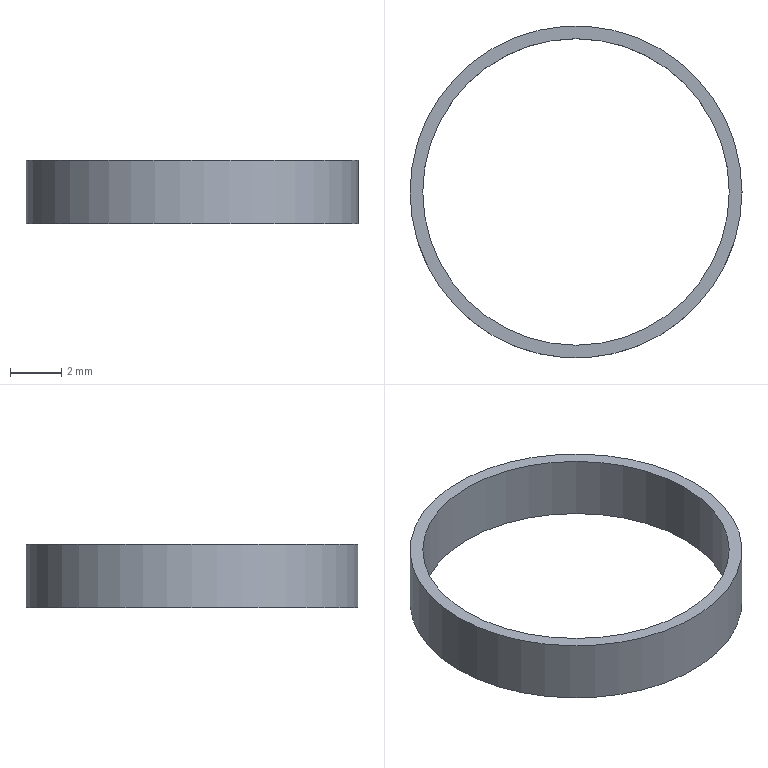Part | STEP file | lll_id1134_x_t | 1 solid | 4 faces | box 13 x 13 x 2.5 mm | volume 49.087 mm3 | cylinder 2 | plane 2 | commonest cylinder face diameters 12 x1 13 x1
STEP:
#1=CARTESIAN_POINT('',(383.,-100.,-0.15));
#2=VERTEX_POINT('',#1);
#3=CARTESIAN_POINT('',(389.5,-100.,-0.15));
#4=DIRECTION('',(0.,0.,1.));
#5=DIRECTION('',(-1.,0.,0.));
#6=AXIS2_PLACEMENT_3D('',#3,#4,#5);
#7=CIRCLE('',#6,6.5);
#8=EDGE_CURVE('',#2,#2,#7,.T.);
#9=ORIENTED_EDGE('',*,*,#8,.T.);
#10=EDGE_LOOP('',(#9));
#11=FACE_BOUND('',#10,.T.);
#12=CARTESIAN_POINT('',(383.,-100.,2.35));
#13=VERTEX_POINT('',#12);
#14=CARTESIAN_POINT('',(389.5,-100.,2.35));
#15=DIRECTION('',(0.,0.,1.));
#16=DIRECTION('',(-1.,0.,0.));
#17=AXIS2_PLACEMENT_3D('',#14,#15,#16);
#18=CIRCLE('',#17,6.5);
#19=EDGE_CURVE('',#13,#13,#18,.T.);
#20=ORIENTED_EDGE('',*,*,#19,.F.);
#21=EDGE_LOOP('',(#20));
#22=FACE_BOUND('',#21,.T.);
#23=CARTESIAN_POINT('',(389.5,-100.,-0.15));
#24=DIRECTION('',(0.,0.,1.));
#25=DIRECTION('',(1.,0.,0.));
#26=AXIS2_PLACEMENT_3D('',#23,#24,#25);
#27=CYLINDRICAL_SURFACE('',#26,6.5);
#28=ADVANCED_FACE('',(#11,#22),#27,.T.);
#29=CARTESIAN_POINT('',(383.5,-100.,-0.15));
#30=VERTEX_POINT('',#29);
#31=CARTESIAN_POINT('',(389.5,-100.,-0.15));
#32=DIRECTION('',(0.,0.,1.));
#33=DIRECTION('',(-1.,0.,0.));
#34=AXIS2_PLACEMENT_3D('',#31,#32,#33);
#35=CIRCLE('',#34,6.);
#36=EDGE_CURVE('',#30,#30,#35,.T.);
#37=ORIENTED_EDGE('',*,*,#36,.F.);
#38=EDGE_LOOP('',(#37));
#39=FACE_BOUND('',#38,.T.);
#40=CARTESIAN_POINT('',(383.5,-100.,2.35));
#41=VERTEX_POINT('',#40);
#42=CARTESIAN_POINT('',(389.5,-100.,2.35));
#43=DIRECTION('',(0.,0.,1.));
#44=DIRECTION('',(-1.,0.,0.));
#45=AXIS2_PLACEMENT_3D('',#42,#43,#44);
#46=CIRCLE('',#45,6.);
#47=EDGE_CURVE('',#41,#41,#46,.T.);
#48=ORIENTED_EDGE('',*,*,#47,.T.);
#49=EDGE_LOOP('',(#48));
#50=FACE_BOUND('',#49,.T.);
#51=CARTESIAN_POINT('',(389.5,-100.,-0.15));
#52=DIRECTION('',(0.,0.,1.));
#53=DIRECTION('',(1.,0.,0.));
#54=AXIS2_PLACEMENT_3D('',#51,#52,#53);
#55=CYLINDRICAL_SURFACE('',#54,6.);
#56=ADVANCED_FACE('',(#39,#50),#55,.F.);
#57=ORIENTED_EDGE('',*,*,#8,.F.);
#58=EDGE_LOOP('',(#57));
#59=FACE_BOUND('',#58,.T.);
#60=ORIENTED_EDGE('',*,*,#36,.T.);
#61=EDGE_LOOP('',(#60));
#62=FACE_BOUND('',#61,.T.);
#63=CARTESIAN_POINT('',(389.5,-100.,-0.15));
#64=DIRECTION('',(0.,0.,1.));
#65=DIRECTION('',(1.,0.,0.));
#66=AXIS2_PLACEMENT_3D('',#63,#64,#65);
#67=PLANE('',#66);
#68=ADVANCED_FACE('',(#59,#62),#67,.F.);
#69=ORIENTED_EDGE('',*,*,#19,.T.);
#70=EDGE_LOOP('',(#69));
#71=FACE_BOUND('',#70,.T.);
#72=ORIENTED_EDGE('',*,*,#47,.F.);
#73=EDGE_LOOP('',(#72));
#74=FACE_BOUND('',#73,.T.);
#75=CARTESIAN_POINT('',(389.5,-100.,2.35));
#76=DIRECTION('',(0.,0.,1.));
#77=DIRECTION('',(1.,0.,0.));
#78=AXIS2_PLACEMENT_3D('',#75,#76,#77);
#79=PLANE('',#78);
#80=ADVANCED_FACE('',(#71,#74),#79,.T.);
#81=CLOSED_SHELL('',(#28,#56,#68,#80));
#82=MANIFOLD_SOLID_BREP('',#81);
#83=(LENGTH_UNIT()NAMED_UNIT(*)SI_UNIT(.MILLI.,.METRE.));
#84=UNCERTAINTY_MEASURE_WITH_UNIT(LENGTH_MEASURE(0.00002),#83,'','');
#85=(NAMED_UNIT(*)PLANE_ANGLE_UNIT()SI_UNIT($,.RADIAN.));
#86=PLANE_ANGLE_MEASURE_WITH_UNIT(PLANE_ANGLE_MEASURE(0.01745),#85);
#87=DIMENSIONAL_EXPONENTS(0.,0.,0.,0.,0.,0.,0.);
#88=(CONVERSION_BASED_UNIT('DEGREE',#86)NAMED_UNIT(#87)PLANE_ANGLE_UNIT());
#89=(NAMED_UNIT(*)SI_UNIT($,.STERADIAN.)SOLID_ANGLE_UNIT());
#90=(GEOMETRIC_REPRESENTATION_CONTEXT(3)GLOBAL_UNCERTAINTY_ASSIGNED_CONTEXT((#84))GLOBAL_UNIT_ASSIGNED_CONTEXT((#83,#88,#89))REPRESENTATION_CONTEXT('',''));
#91=ADVANCED_BREP_SHAPE_REPRESENTATION('',(#82),#90);